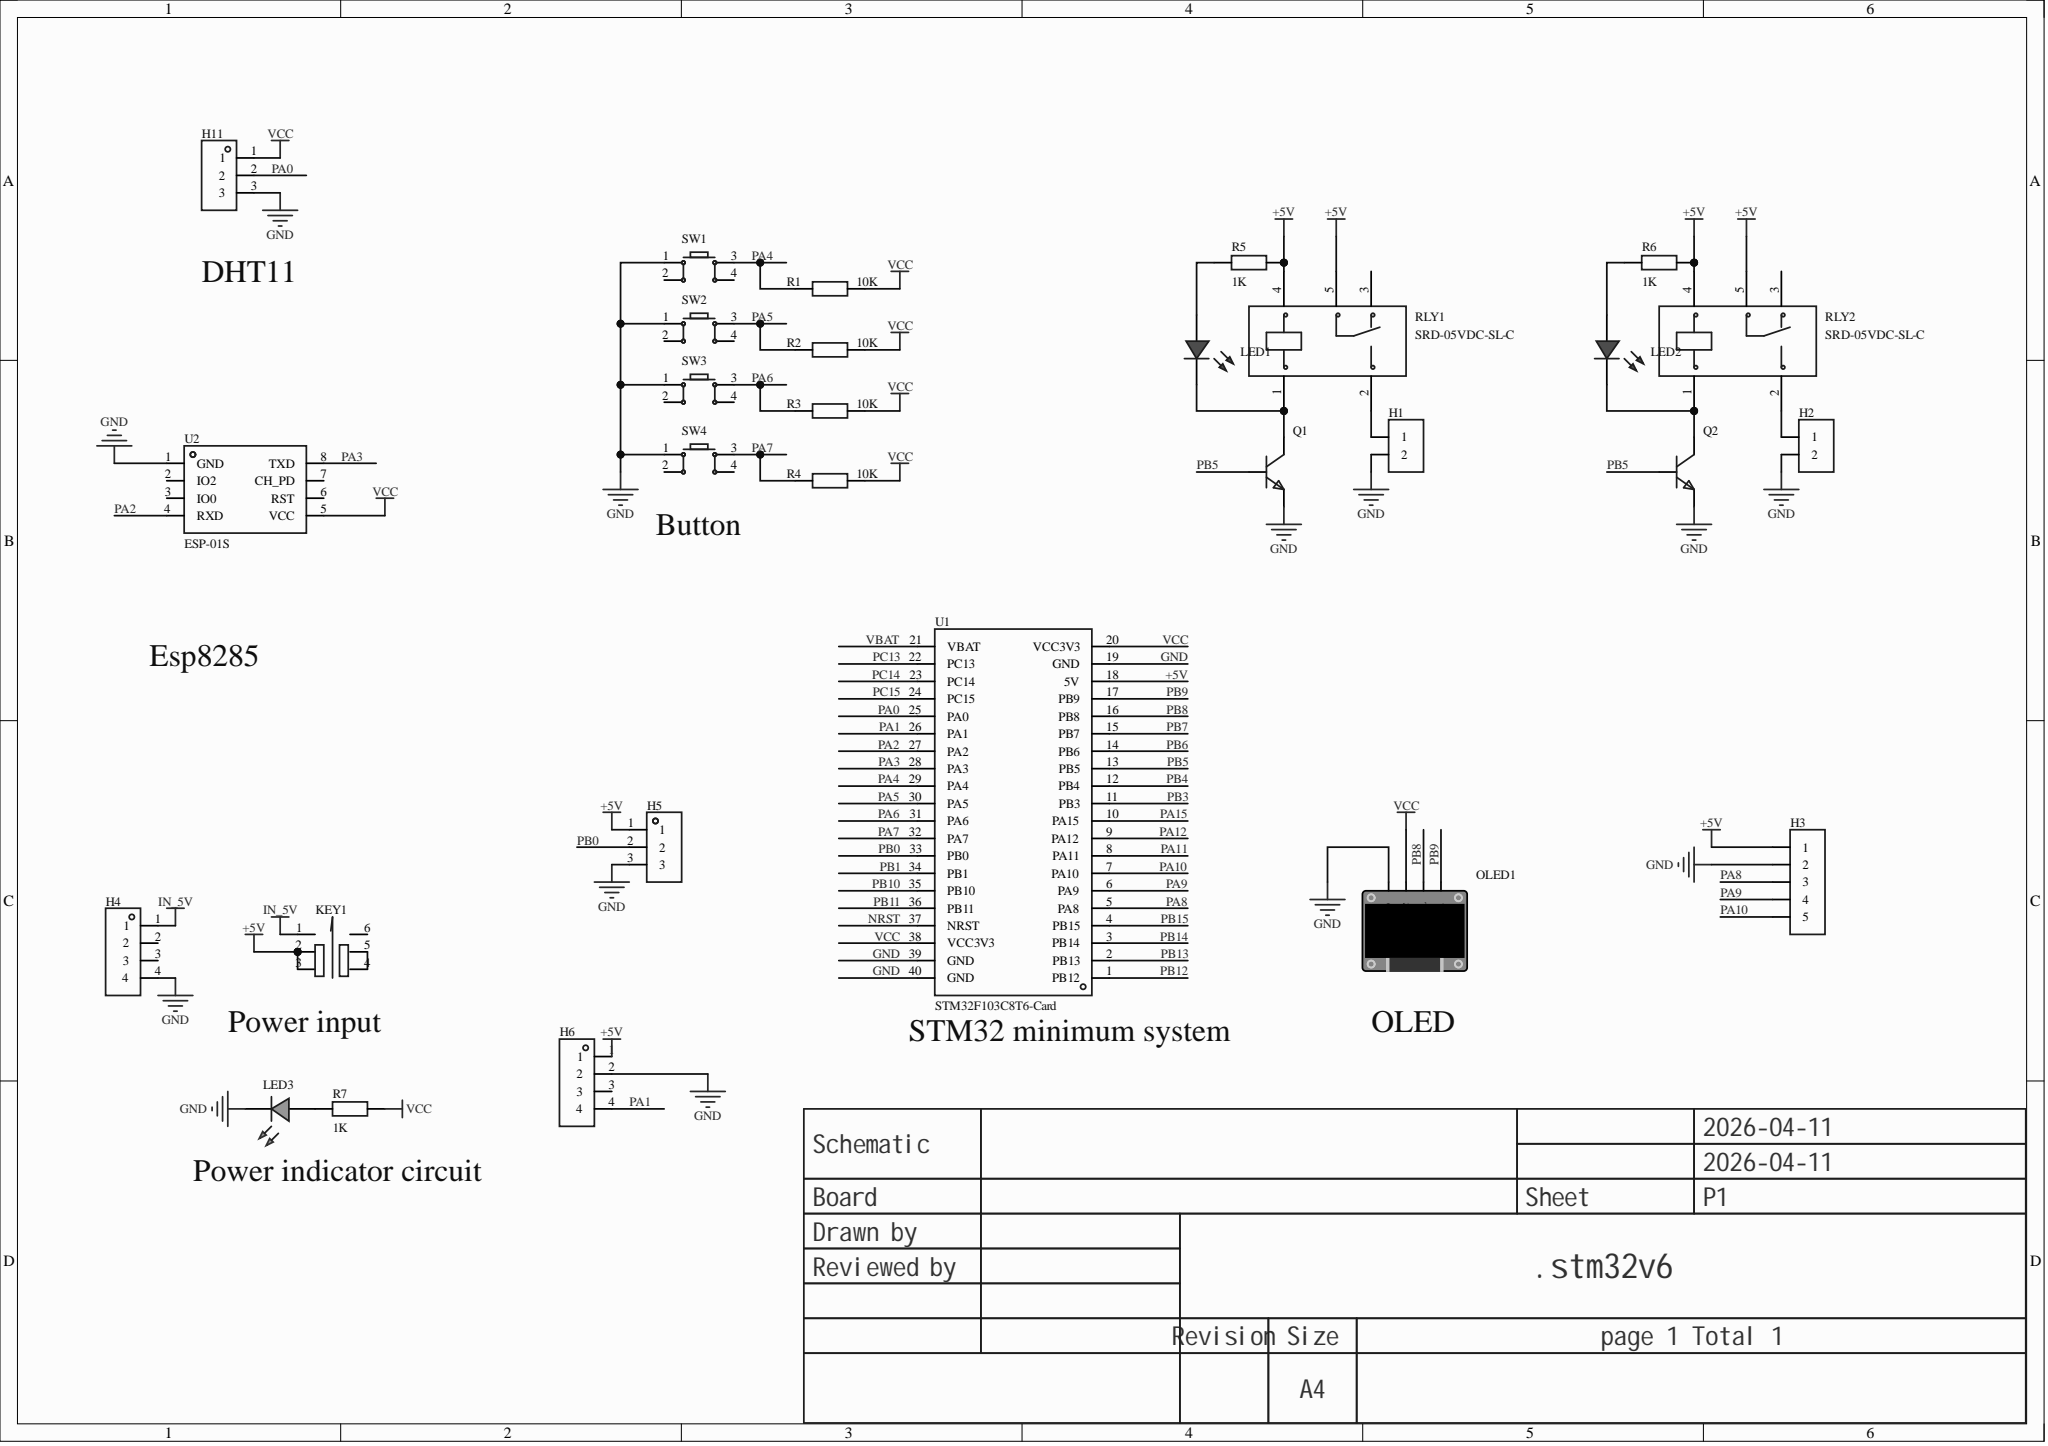Circuit board | Altium Designer | 29 parts | 27 nets
Bill of materials:
Comment,Description,Designator,Footprint,LibRef,Quantity
"","","H1, H2","HDR-TH_2P-P2.54-V-F","HDR-F_2.54_1x2P","2"
"","","H3","HDR-TH_5P-P2.54-V-F","HDR-F_2.54_1x5P","1"
"","","H4, H6","HDR-TH_4P-P2.54-V-F","HDR-F_2.54_1x4P","2"
"","","H5, H11","HDR-TH_3P-P2.54-V-F","HDR-F_2.54_1x3P","2"
"Self-locking switch 5.8Z white-grey-white 260G","","KEY1","SW-TH_6P-L5.8-W5.8-P2.00-LS4.5-TR","自锁开关 5.8Z白灰白260G","1"
"","","LED1, LED2, LED3","LED_TH-3mm","LED_TH-R_3mm, LED_TH-G_3mm","3"
"","","OLED1","0.96OLED_4P","0.96OLED模块_4P","1"
"","","Q1, Q2","S8050_SOT-23","S8050_SOT_NPN","2"
"10K","","R1, R2, R3, R4","R0603","Res_0603","4"
"1K","","R5, R6, R7","R0603","Res_0603","3"
"SRD-05VDC-SL-C","Coil voltage:5V;Contact form:One changeover:1C (SPDT);Contact rating (resistive load):-;Max switching voltage:250V@AC;Max switching current:15A;","RLY1, RLY2","RELAY-TH_SRD-XXVDC-XL-C","SRD-05VDC-SL-C","2"
"","","SW1, SW2, SW3, SW4","SW-TH_4P-L6.0-W6.0-P4.50-LS6.5","Key_TH_6x6x6","4"
"STM32F103C8T6-Card","","U1","CONN-TH_L53.3-W22.9_STM32F103C8T6-CARD","STM32F103C8T6-Card","1"
"ESP-01S","","U2","WIFIM-TH_ESP-01S","ESP-01S_C111009","1"
Netlist (Protel format):
[
H1
HDR-TH_2P-P2.54-V-F




]
[
H2
HDR-TH_2P-P2.54-V-F




]
[
H3
HDR-TH_5P-P2.54-V-F




]
[
H4
HDR-TH_4P-P2.54-V-F




]
[
H5
HDR-TH_3P-P2.54-V-F




]
[
H6
HDR-TH_4P-P2.54-V-F




]
[
H11
HDR-TH_3P-P2.54-V-F




]
[
KEY1
SW-TH_6P-L5.8-W5.8-P2.00-LS4.5-TR
Self-locking switch 5.8Z white-grey-white 260G



]
[
LED1
LED_TH-3mm




]
[
LED2
LED_TH-3mm




]
[
LED3
LED_TH-3mm




]
[
OLED1
0.96OLED_4P




]
[
Q1
S8050_SOT-23




]
[
Q2
S8050_SOT-23




]
[
R1
R0603
10K



]
[
R2
R0603
10K



]
[
R3
R0603
10K



]
[
R4
R0603
10K



]
[
R5
R0603
1K



]
[
R6
R0603
1K



]
[
R7
R0603
1K



]
[
RLY1
RELAY-TH_SRD-XXVDC-XL-C
SRD-05VDC-SL-C



]
[
RLY2
RELAY-TH_SRD-XXVDC-XL-C
SRD-05VDC-SL-C



]
[
SW1
SW-TH_4P-L6.0-W6.0-P4.50-LS6.5




]
[
SW2
SW-TH_4P-L6.0-W6.0-P4.50-LS6.5




]
[
SW3
SW-TH_4P-L6.0-W6.0-P4.50-LS6.5




]
[
SW4
SW-TH_4P-L6.0-W6.0-P4.50-LS6.5




]
[
U1
CONN-TH_L53.3-W22.9_STM32F103C8T6-CARD
STM32F103C8T6-Card



]
[
U2
WIFIM-TH_ESP-01S
ESP-01S



]
(
VCC
H11-1
OLED1-2
R1-2
R2-2
R3-2
R4-2
R7-2
U1-20
U1-38
U2-5
)
(
PB9
OLED1-4
U1-17
)
(
PB8
OLED1-3
U1-16
)
(
PB5
Q1-1
Q2-1
U1-13
)
(
PB0
H5-2
U1-33
)
(
PA10
H3-5
U1-7
)
(
PA9
H3-4
U1-6
)
(
PA8
H3-3
U1-5
)
(
PA7
R4-1
SW4-3
U1-32
)
(
PA6
R3-1
SW3-3
U1-31
)
(
PA5
R2-1
SW2-3
U1-30
)
(
PA4
R1-1
SW1-3
U1-29
)
(
PA3
U1-28
U2-8
)
(
PA2
U1-27
U2-4
)
(
PA1
H6-4
U1-26
)
(
PA0
H11-2
U1-25
)
(
NetLED3_1
LED3-1
R7-1
)
(
NetLED2_2
LED2-2
Q2-3
RLY2-1
)
(
NetLED2_1
LED2-1
R6-1
)
(
NetLED1_2
LED1-2
Q1-3
RLY1-1
)
(
NetLED1_1
LED1-1
R5-1
)
(
NetKEY1_4
KEY1-4
KEY1-5
)
(
NetH2_1
H2-1
RLY2-2
)
(
NetH1_1
H1-1
RLY1-2
)
(
IN_5V
H4-1
KEY1-1
)
(
GND
H1-2
H2-2
H3-2
H4-4
H5-3
H6-2
H11-3
LED3-2
OLED1-1
Q1-2
Q2-2
SW1-1
SW2-1
SW3-1
SW4-1
U1-19
U1-39
U1-40
U2-1
)
(
+5V
H3-1
H5-1
H6-1
KEY1-2
KEY1-3
R5-2
R6-2
RLY1-4
RLY1-5
RLY2-4
RLY2-5
U1-18
)